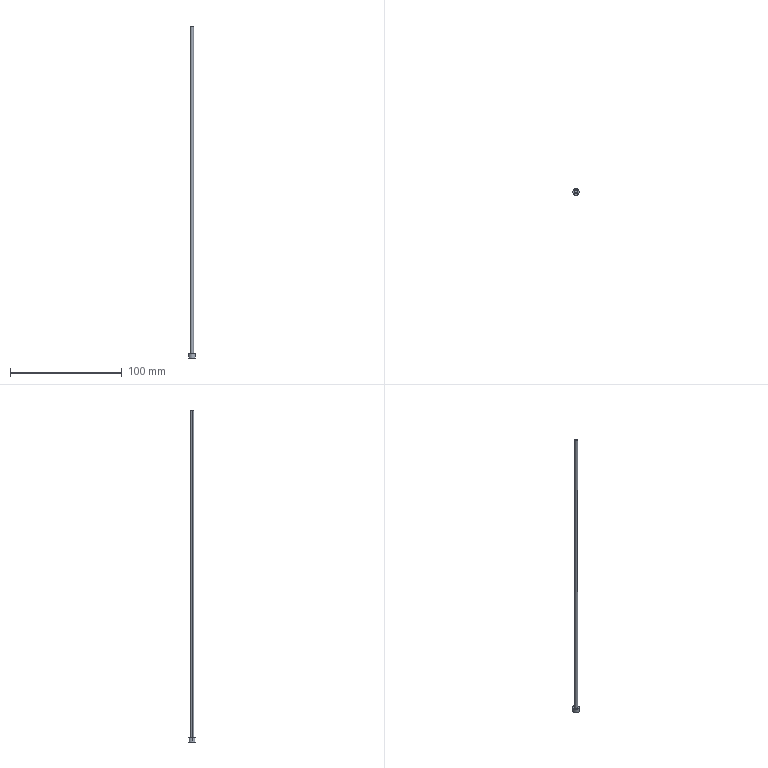Part | Creo | 1 solid | 7 faces | box 6 x 6 x 297.407 mm | volume 2187 mm3 | cylinder 4 | plane 3 | commonest cylinder face diameters 3 x2 6 x2
STEP:
#1=CARTESIAN_POINT('',(57.3,-73.,1.407));
#2=VERTEX_POINT('',#1);
#3=CARTESIAN_POINT('',(54.3,-73.,1.407));
#4=VERTEX_POINT('',#3);
#5=CARTESIAN_POINT('',(55.8,-73.,1.407));
#6=DIRECTION('',(0.,0.,1.));
#7=DIRECTION('',(1.,0.,0.));
#8=AXIS2_PLACEMENT_3D('',#5,#6,#7);
#9=CIRCLE('',#8,1.5);
#10=EDGE_CURVE('',#2,#4,#9,.T.);
#11=ORIENTED_EDGE('',*,*,#10,.F.);
#12=CARTESIAN_POINT('',(55.8,-73.,1.407));
#13=DIRECTION('',(0.,0.,1.));
#14=DIRECTION('',(-1.,0.,0.));
#15=AXIS2_PLACEMENT_3D('',#12,#13,#14);
#16=CIRCLE('',#15,1.5);
#17=EDGE_CURVE('',#4,#2,#16,.T.);
#18=ORIENTED_EDGE('',*,*,#17,.F.);
#19=EDGE_LOOP('',(#11,#18));
#20=FACE_OUTER_BOUND('',#19,.F.);
#21=CARTESIAN_POINT('',(-0.2,-0.0754,1.407));
#22=DIRECTION('',(0.,0.,1.));
#23=DIRECTION('',(0.,-1.,0.));
#24=AXIS2_PLACEMENT_3D('',#21,#22,#23);
#25=PLANE('',#24);
#26=ADVANCED_FACE('',(#20),#25,.T.);
#27=CARTESIAN_POINT('',(54.3,-73.,-292.));
#28=VERTEX_POINT('',#27);
#29=CARTESIAN_POINT('',(57.3,-73.,-292.));
#30=VERTEX_POINT('',#29);
#31=CARTESIAN_POINT('',(55.8,-73.,-292.));
#32=DIRECTION('',(0.,0.,-1.));
#33=DIRECTION('',(-1.,0.,0.));
#34=AXIS2_PLACEMENT_3D('',#31,#32,#33);
#35=CIRCLE('',#34,1.5);
#36=EDGE_CURVE('',#28,#30,#35,.T.);
#37=ORIENTED_EDGE('',*,*,#36,.T.);
#38=CARTESIAN_POINT('',(57.3,-73.,-292.));
#39=DIRECTION('',(0.,0.,1.));
#40=VECTOR('',#39,293.407);
#41=LINE('',#38,#40);
#42=EDGE_CURVE('',#30,#2,#41,.T.);
#43=ORIENTED_EDGE('',*,*,#42,.T.);
#44=ORIENTED_EDGE('',*,*,#10,.T.);
#45=CARTESIAN_POINT('',(54.3,-73.,-292.));
#46=DIRECTION('',(0.,0.,1.));
#47=VECTOR('',#46,293.407);
#48=LINE('',#45,#47);
#49=EDGE_CURVE('',#28,#4,#48,.T.);
#50=ORIENTED_EDGE('',*,*,#49,.F.);
#51=EDGE_LOOP('',(#37,#43,#44,#50));
#52=FACE_OUTER_BOUND('',#51,.F.);
#53=CARTESIAN_POINT('',(55.8,-73.,-352.221));
#54=DIRECTION('',(0.,0.,1.));
#55=DIRECTION('',(1.,0.,0.));
#56=AXIS2_PLACEMENT_3D('',#53,#54,#55);
#57=CYLINDRICAL_SURFACE('',#56,1.5);
#58=ADVANCED_FACE('',(#52),#57,.T.);
#59=CARTESIAN_POINT('',(58.8,-73.,-292.));
#60=VERTEX_POINT('',#59);
#61=CARTESIAN_POINT('',(52.8,-73.,-292.));
#62=VERTEX_POINT('',#61);
#63=CARTESIAN_POINT('',(55.8,-73.,-292.));
#64=DIRECTION('',(0.,0.,1.));
#65=DIRECTION('',(1.,0.,0.));
#66=AXIS2_PLACEMENT_3D('',#63,#64,#65);
#67=CIRCLE('',#66,3.);
#68=EDGE_CURVE('',#60,#62,#67,.T.);
#69=ORIENTED_EDGE('',*,*,#68,.F.);
#70=CARTESIAN_POINT('',(55.8,-73.,-292.));
#71=DIRECTION('',(0.,0.,1.));
#72=DIRECTION('',(-1.,0.,0.));
#73=AXIS2_PLACEMENT_3D('',#70,#71,#72);
#74=CIRCLE('',#73,3.);
#75=EDGE_CURVE('',#62,#60,#74,.T.);
#76=ORIENTED_EDGE('',*,*,#75,.F.);
#77=EDGE_LOOP('',(#69,#76));
#78=FACE_OUTER_BOUND('',#77,.F.);
#79=CARTESIAN_POINT('',(55.8,-73.,-292.));
#80=DIRECTION('',(0.,0.,-1.));
#81=DIRECTION('',(1.,0.,0.));
#82=AXIS2_PLACEMENT_3D('',#79,#80,#81);
#83=CIRCLE('',#82,1.5);
#84=EDGE_CURVE('',#30,#28,#83,.T.);
#85=ORIENTED_EDGE('',*,*,#84,.F.);
#86=ORIENTED_EDGE('',*,*,#36,.F.);
#87=EDGE_LOOP('',(#85,#86));
#88=FACE_BOUND('',#87,.F.);
#89=CARTESIAN_POINT('',(55.8,-73.,-292.));
#90=DIRECTION('',(0.,0.,1.));
#91=DIRECTION('',(-1.,0.,0.));
#92=AXIS2_PLACEMENT_3D('',#89,#90,#91);
#93=PLANE('',#92);
#94=ADVANCED_FACE('',(#78,#88),#93,.T.);
#95=ORIENTED_EDGE('',*,*,#84,.T.);
#96=ORIENTED_EDGE('',*,*,#49,.T.);
#97=ORIENTED_EDGE('',*,*,#17,.T.);
#98=ORIENTED_EDGE('',*,*,#42,.F.);
#99=EDGE_LOOP('',(#95,#96,#97,#98));
#100=FACE_OUTER_BOUND('',#99,.F.);
#101=CARTESIAN_POINT('',(55.8,-73.,-352.221));
#102=DIRECTION('',(0.,0.,1.));
#103=DIRECTION('',(1.,0.,0.));
#104=AXIS2_PLACEMENT_3D('',#101,#102,#103);
#105=CYLINDRICAL_SURFACE('',#104,1.5);
#106=ADVANCED_FACE('',(#100),#105,.T.);
#107=ORIENTED_EDGE('',*,*,#68,.T.);
#108=CARTESIAN_POINT('',(52.8,-73.,-296.));
#109=VERTEX_POINT('',#108);
#110=CARTESIAN_POINT('',(52.8,-73.,-296.));
#111=DIRECTION('',(0.,0.,1.));
#112=VECTOR('',#111,4.);
#113=LINE('',#110,#112);
#114=EDGE_CURVE('',#109,#62,#113,.T.);
#115=ORIENTED_EDGE('',*,*,#114,.F.);
#116=CARTESIAN_POINT('',(58.8,-73.,-296.));
#117=VERTEX_POINT('',#116);
#118=CARTESIAN_POINT('',(55.8,-73.,-296.));
#119=DIRECTION('',(0.,0.,-1.));
#120=DIRECTION('',(-1.,0.,0.));
#121=AXIS2_PLACEMENT_3D('',#118,#119,#120);
#122=CIRCLE('',#121,3.);
#123=EDGE_CURVE('',#109,#117,#122,.T.);
#124=ORIENTED_EDGE('',*,*,#123,.T.);
#125=CARTESIAN_POINT('',(58.8,-73.,-296.));
#126=DIRECTION('',(0.,0.,1.));
#127=VECTOR('',#126,4.);
#128=LINE('',#125,#127);
#129=EDGE_CURVE('',#117,#60,#128,.T.);
#130=ORIENTED_EDGE('',*,*,#129,.T.);
#131=EDGE_LOOP('',(#107,#115,#124,#130));
#132=FACE_OUTER_BOUND('',#131,.F.);
#133=CARTESIAN_POINT('',(55.8,-73.,-296.));
#134=DIRECTION('',(0.,0.,1.));
#135=DIRECTION('',(-1.,0.,0.));
#136=AXIS2_PLACEMENT_3D('',#133,#134,#135);
#137=CYLINDRICAL_SURFACE('',#136,3.);
#138=ADVANCED_FACE('',(#132),#137,.T.);
#139=ORIENTED_EDGE('',*,*,#75,.T.);
#140=ORIENTED_EDGE('',*,*,#129,.F.);
#141=CARTESIAN_POINT('',(55.8,-73.,-296.));
#142=DIRECTION('',(0.,0.,-1.));
#143=DIRECTION('',(1.,0.,0.));
#144=AXIS2_PLACEMENT_3D('',#141,#142,#143);
#145=CIRCLE('',#144,3.);
#146=EDGE_CURVE('',#117,#109,#145,.T.);
#147=ORIENTED_EDGE('',*,*,#146,.T.);
#148=ORIENTED_EDGE('',*,*,#114,.T.);
#149=EDGE_LOOP('',(#139,#140,#147,#148));
#150=FACE_OUTER_BOUND('',#149,.F.);
#151=CARTESIAN_POINT('',(55.8,-73.,-296.));
#152=DIRECTION('',(0.,0.,1.));
#153=DIRECTION('',(-1.,0.,0.));
#154=AXIS2_PLACEMENT_3D('',#151,#152,#153);
#155=CYLINDRICAL_SURFACE('',#154,3.);
#156=ADVANCED_FACE('',(#150),#155,.T.);
#157=ORIENTED_EDGE('',*,*,#146,.F.);
#158=ORIENTED_EDGE('',*,*,#123,.F.);
#159=EDGE_LOOP('',(#157,#158));
#160=FACE_OUTER_BOUND('',#159,.F.);
#161=CARTESIAN_POINT('',(10.,-0.0801,-296.));
#162=DIRECTION('',(0.,0.,1.));
#163=DIRECTION('',(0.,1.,0.));
#164=AXIS2_PLACEMENT_3D('',#161,#162,#163);
#165=PLANE('',#164);
#166=ADVANCED_FACE('',(#160),#165,.F.);
#167=CLOSED_SHELL('',(#26,#58,#94,#106,#138,#156,#166));
#168=MANIFOLD_SOLID_BREP('',#167);
#169=(LENGTH_UNIT()NAMED_UNIT(*)SI_UNIT(.MILLI.,.METRE.));
#170=UNCERTAINTY_MEASURE_WITH_UNIT(LENGTH_MEASURE(0.02975),#169,'','');
#171=(NAMED_UNIT(*)PLANE_ANGLE_UNIT()SI_UNIT($,.RADIAN.));
#172=PLANE_ANGLE_MEASURE_WITH_UNIT(PLANE_ANGLE_MEASURE(0.01745),#171);
#173=(CONVERSION_BASED_UNIT('DEGREE',#172)NAMED_UNIT(*)PLANE_ANGLE_UNIT());
#174=(NAMED_UNIT(*)SI_UNIT($,.STERADIAN.)SOLID_ANGLE_UNIT());
#175=(GEOMETRIC_REPRESENTATION_CONTEXT(3)GLOBAL_UNCERTAINTY_ASSIGNED_CONTEXT((#170))GLOBAL_UNIT_ASSIGNED_CONTEXT((#169,#173,#174))REPRESENTATION_CONTEXT('',''));
#176=ADVANCED_BREP_SHAPE_REPRESENTATION('',(#168),#175);